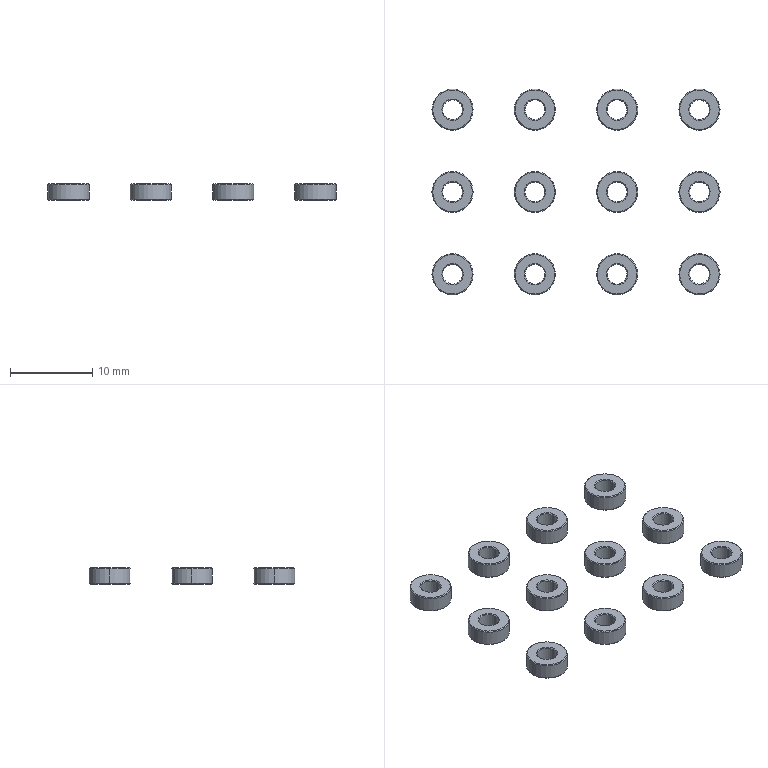NC program | NX | posted with a generic post | part box 35 x 25 x 2 mm
Lines 1 to 47 of 5177:
N10 G17 G21 G94 G90
(DRILLING , TOOL : D6A45)
N12 T07 M6
N14 G54
N16 G17 G0 G90 X32.5 Y22.5 S5000 M3
N18 G43 Z30. H7
N20 G94 G81 G98 Z-1.3 F250. R3.
N22 Y12.5
N24 Y2.5
N26 X22.5
N28 X12.5
N30 X2.5
N32 Y12.5
N34 Y22.5
N36 X12.5
N38 X22.5
N40 Y12.5
N42 X12.5
N44 G80
N46 G0 X12.5 Y12.5 Z30.
N48 M5
(DRILLING_COPY , TOOL : 2.4ZT)
N50 T14 M6
N52 G54
N54 G17 G0 G90 X32.5 Y12.5 S2000 M3
N56 G43 Z30. H14
N58 G94 G83 G98 Z-4.221 F150. Q2. R3.
N60 Y2.5
N62 X22.5
N64 Y12.5
N66 X12.5
N68 Y2.5
N70 X2.5
N72 Y12.5
N74 Y22.5
N76 X12.5
N78 X22.5
N80 X32.5
N82 G80
N84 G0 X32.5 Y22.5 Z30.
N86 M5